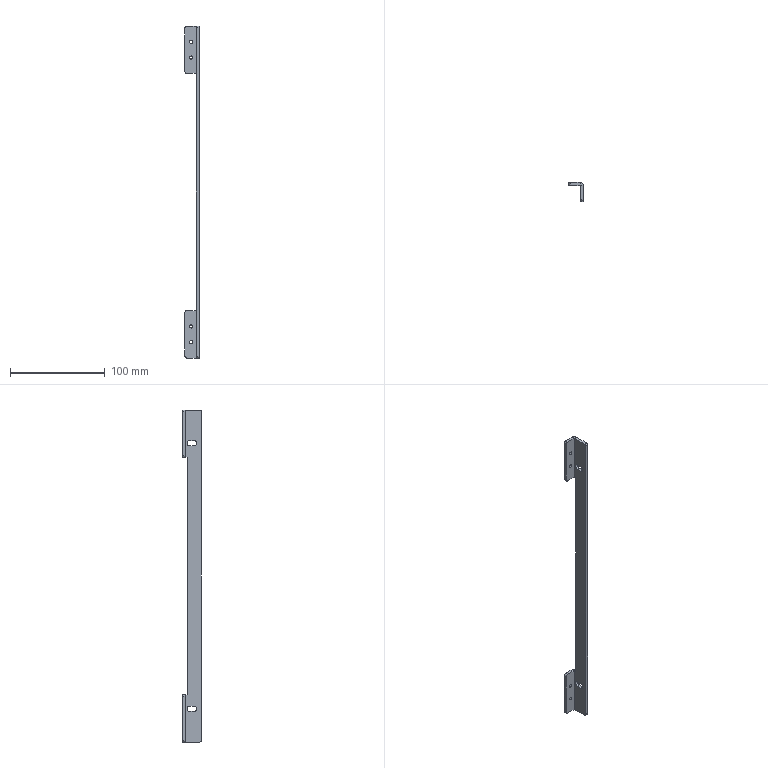Part | STEP file | 1 solid | 50 faces | box 15 x 20 x 350 mm | volume 20205 mm3 | plane 26 | cylinder 24 | commonest cylinder face diameters 3.3 x8 4 x6 5.5 x6 0.4 x2 6.4 x2